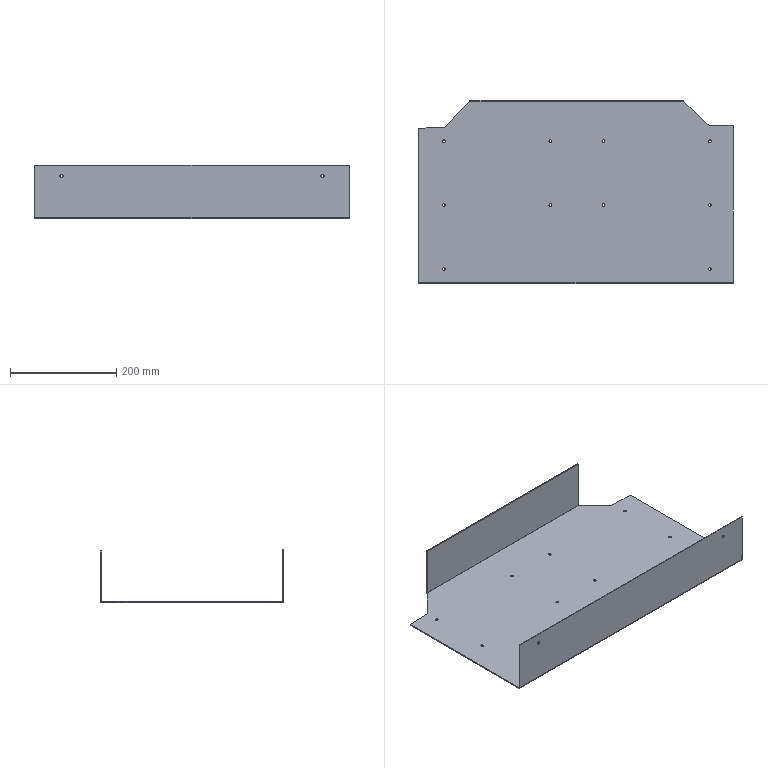Part | STEP file | Assembly TS-001-01 | 1 solid | 52 faces | box 590.5 x 344 x 100 mm | volume 582857 mm3 | cylinder 28 | plane 24 | commonest cylinder face diameters 5 x20 6 x4 0.4 x2 4.4 x2